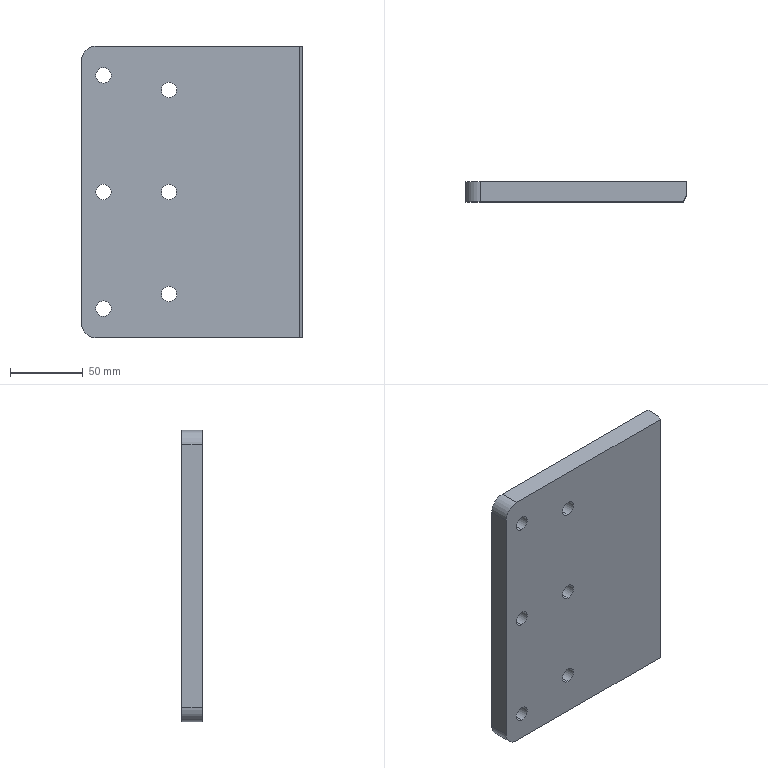Part | SolidWorks | features HoleWzd 2, ICE 2, Extrusion 1, Fillet 1 | 1 solid | 21 faces | box 151.5 x 14 x 200 mm | volume 415411 mm3 | cylinder 14 | plane 7 | commonest cylinder face diameters 10.5 x12 20 x2
STEP:
#1=CARTESIAN_POINT('',(15.,0.,-85.25));
#2=VERTEX_POINT('',#1);
#3=CARTESIAN_POINT('',(15.,0.,-74.75));
#4=VERTEX_POINT('',#3);
#5=CARTESIAN_POINT('',(15.,0.,-80.));
#6=DIRECTION('',(0.,1.,0.));
#7=DIRECTION('',(0.,0.,1.));
#8=AXIS2_PLACEMENT_3D('',#5,#6,#7);
#9=CIRCLE('',#8,5.25);
#10=EDGE_CURVE('',#2,#4,#9,.T.);
#11=ORIENTED_EDGE('',*,*,#10,.F.);
#12=CARTESIAN_POINT('',(15.,14.,-85.25));
#13=VERTEX_POINT('',#12);
#14=CARTESIAN_POINT('',(15.,14.,-85.25));
#15=DIRECTION('',(0.,1.,0.));
#16=VECTOR('',#15,1000.);
#17=LINE('',#14,#16);
#18=EDGE_CURVE('',#2,#13,#17,.T.);
#19=ORIENTED_EDGE('',*,*,#18,.T.);
#20=CARTESIAN_POINT('',(15.,14.,-74.75));
#21=VERTEX_POINT('',#20);
#22=CARTESIAN_POINT('',(15.,14.,-80.));
#23=DIRECTION('',(0.,1.,0.));
#24=DIRECTION('',(0.,0.,1.));
#25=AXIS2_PLACEMENT_3D('',#22,#23,#24);
#26=CIRCLE('',#25,5.25);
#27=EDGE_CURVE('',#13,#21,#26,.T.);
#28=ORIENTED_EDGE('',*,*,#27,.T.);
#29=CARTESIAN_POINT('',(15.,14.,-74.75));
#30=DIRECTION('',(0.,1.,0.));
#31=VECTOR('',#30,1000.);
#32=LINE('',#29,#31);
#33=EDGE_CURVE('',#4,#21,#32,.T.);
#34=ORIENTED_EDGE('',*,*,#33,.F.);
#35=EDGE_LOOP('',(#11,#19,#28,#34));
#36=FACE_OUTER_BOUND('',#35,.T.);
#37=CARTESIAN_POINT('',(15.,14.,-80.));
#38=DIRECTION('',(0.,1.,0.));
#39=DIRECTION('',(0.,0.,1.));
#40=AXIS2_PLACEMENT_3D('',#37,#38,#39);
#41=CYLINDRICAL_SURFACE('',#40,5.25);
#42=ADVANCED_FACE('',(#36),#41,.F.);
#43=CARTESIAN_POINT('',(15.,0.,74.75));
#44=VERTEX_POINT('',#43);
#45=CARTESIAN_POINT('',(15.,0.,85.25));
#46=VERTEX_POINT('',#45);
#47=CARTESIAN_POINT('',(15.,0.,80.));
#48=DIRECTION('',(0.,1.,0.));
#49=DIRECTION('',(0.,0.,1.));
#50=AXIS2_PLACEMENT_3D('',#47,#48,#49);
#51=CIRCLE('',#50,5.25);
#52=EDGE_CURVE('',#44,#46,#51,.T.);
#53=ORIENTED_EDGE('',*,*,#52,.F.);
#54=CARTESIAN_POINT('',(15.,14.,74.75));
#55=VERTEX_POINT('',#54);
#56=CARTESIAN_POINT('',(15.,14.,74.75));
#57=DIRECTION('',(0.,1.,0.));
#58=VECTOR('',#57,1000.);
#59=LINE('',#56,#58);
#60=EDGE_CURVE('',#44,#55,#59,.T.);
#61=ORIENTED_EDGE('',*,*,#60,.T.);
#62=CARTESIAN_POINT('',(15.,14.,85.25));
#63=VERTEX_POINT('',#62);
#64=CARTESIAN_POINT('',(15.,14.,80.));
#65=DIRECTION('',(0.,1.,0.));
#66=DIRECTION('',(0.,0.,1.));
#67=AXIS2_PLACEMENT_3D('',#64,#65,#66);
#68=CIRCLE('',#67,5.25);
#69=EDGE_CURVE('',#55,#63,#68,.T.);
#70=ORIENTED_EDGE('',*,*,#69,.T.);
#71=CARTESIAN_POINT('',(15.,14.,85.25));
#72=DIRECTION('',(0.,1.,0.));
#73=VECTOR('',#72,1000.);
#74=LINE('',#71,#73);
#75=EDGE_CURVE('',#46,#63,#74,.T.);
#76=ORIENTED_EDGE('',*,*,#75,.F.);
#77=EDGE_LOOP('',(#53,#61,#70,#76));
#78=FACE_OUTER_BOUND('',#77,.T.);
#79=CARTESIAN_POINT('',(15.,14.,80.));
#80=DIRECTION('',(0.,1.,0.));
#81=DIRECTION('',(0.,0.,1.));
#82=AXIS2_PLACEMENT_3D('',#79,#80,#81);
#83=CYLINDRICAL_SURFACE('',#82,5.25);
#84=ADVANCED_FACE('',(#78),#83,.F.);
#85=CARTESIAN_POINT('',(15.,0.,-5.25));
#86=VERTEX_POINT('',#85);
#87=CARTESIAN_POINT('',(15.,0.,5.25));
#88=VERTEX_POINT('',#87);
#89=CARTESIAN_POINT('',(15.,0.,0.));
#90=DIRECTION('',(0.,1.,0.));
#91=DIRECTION('',(0.,0.,1.));
#92=AXIS2_PLACEMENT_3D('',#89,#90,#91);
#93=CIRCLE('',#92,5.25);
#94=EDGE_CURVE('',#86,#88,#93,.T.);
#95=ORIENTED_EDGE('',*,*,#94,.F.);
#96=CARTESIAN_POINT('',(15.,14.,-5.25));
#97=VERTEX_POINT('',#96);
#98=CARTESIAN_POINT('',(15.,14.,-5.25));
#99=DIRECTION('',(0.,1.,0.));
#100=VECTOR('',#99,1000.);
#101=LINE('',#98,#100);
#102=EDGE_CURVE('',#86,#97,#101,.T.);
#103=ORIENTED_EDGE('',*,*,#102,.T.);
#104=CARTESIAN_POINT('',(15.,14.,5.25));
#105=VERTEX_POINT('',#104);
#106=CARTESIAN_POINT('',(15.,14.,0.));
#107=DIRECTION('',(0.,1.,0.));
#108=DIRECTION('',(0.,0.,1.));
#109=AXIS2_PLACEMENT_3D('',#106,#107,#108);
#110=CIRCLE('',#109,5.25);
#111=EDGE_CURVE('',#97,#105,#110,.T.);
#112=ORIENTED_EDGE('',*,*,#111,.T.);
#113=CARTESIAN_POINT('',(15.,14.,5.25));
#114=DIRECTION('',(0.,1.,0.));
#115=VECTOR('',#114,1000.);
#116=LINE('',#113,#115);
#117=EDGE_CURVE('',#88,#105,#116,.T.);
#118=ORIENTED_EDGE('',*,*,#117,.F.);
#119=EDGE_LOOP('',(#95,#103,#112,#118));
#120=FACE_OUTER_BOUND('',#119,.T.);
#121=CARTESIAN_POINT('',(15.,14.,0.));
#122=DIRECTION('',(0.,1.,0.));
#123=DIRECTION('',(0.,0.,1.));
#124=AXIS2_PLACEMENT_3D('',#121,#122,#123);
#125=CYLINDRICAL_SURFACE('',#124,5.25);
#126=ADVANCED_FACE('',(#120),#125,.F.);
#127=CARTESIAN_POINT('',(60.,0.,-75.25));
#128=VERTEX_POINT('',#127);
#129=CARTESIAN_POINT('',(60.,0.,-64.75));
#130=VERTEX_POINT('',#129);
#131=CARTESIAN_POINT('',(60.,0.,-70.));
#132=DIRECTION('',(0.,1.,0.));
#133=DIRECTION('',(0.,0.,1.));
#134=AXIS2_PLACEMENT_3D('',#131,#132,#133);
#135=CIRCLE('',#134,5.25);
#136=EDGE_CURVE('',#128,#130,#135,.T.);
#137=ORIENTED_EDGE('',*,*,#136,.F.);
#138=CARTESIAN_POINT('',(60.,14.,-75.25));
#139=VERTEX_POINT('',#138);
#140=CARTESIAN_POINT('',(60.,14.,-75.25));
#141=DIRECTION('',(0.,1.,0.));
#142=VECTOR('',#141,1000.);
#143=LINE('',#140,#142);
#144=EDGE_CURVE('',#128,#139,#143,.T.);
#145=ORIENTED_EDGE('',*,*,#144,.T.);
#146=CARTESIAN_POINT('',(60.,14.,-64.75));
#147=VERTEX_POINT('',#146);
#148=CARTESIAN_POINT('',(60.,14.,-70.));
#149=DIRECTION('',(0.,1.,0.));
#150=DIRECTION('',(0.,0.,1.));
#151=AXIS2_PLACEMENT_3D('',#148,#149,#150);
#152=CIRCLE('',#151,5.25);
#153=EDGE_CURVE('',#139,#147,#152,.T.);
#154=ORIENTED_EDGE('',*,*,#153,.T.);
#155=CARTESIAN_POINT('',(60.,14.,-64.75));
#156=DIRECTION('',(0.,1.,0.));
#157=VECTOR('',#156,1000.);
#158=LINE('',#155,#157);
#159=EDGE_CURVE('',#130,#147,#158,.T.);
#160=ORIENTED_EDGE('',*,*,#159,.F.);
#161=EDGE_LOOP('',(#137,#145,#154,#160));
#162=FACE_OUTER_BOUND('',#161,.T.);
#163=CARTESIAN_POINT('',(60.,14.,-70.));
#164=DIRECTION('',(0.,1.,0.));
#165=DIRECTION('',(0.,0.,1.));
#166=AXIS2_PLACEMENT_3D('',#163,#164,#165);
#167=CYLINDRICAL_SURFACE('',#166,5.25);
#168=ADVANCED_FACE('',(#162),#167,.F.);
#169=CARTESIAN_POINT('',(60.,0.,64.75));
#170=VERTEX_POINT('',#169);
#171=CARTESIAN_POINT('',(60.,0.,75.25));
#172=VERTEX_POINT('',#171);
#173=CARTESIAN_POINT('',(60.,0.,70.));
#174=DIRECTION('',(0.,1.,0.));
#175=DIRECTION('',(0.,0.,1.));
#176=AXIS2_PLACEMENT_3D('',#173,#174,#175);
#177=CIRCLE('',#176,5.25);
#178=EDGE_CURVE('',#170,#172,#177,.T.);
#179=ORIENTED_EDGE('',*,*,#178,.F.);
#180=CARTESIAN_POINT('',(60.,14.,64.75));
#181=VERTEX_POINT('',#180);
#182=CARTESIAN_POINT('',(60.,14.,64.75));
#183=DIRECTION('',(0.,1.,0.));
#184=VECTOR('',#183,1000.);
#185=LINE('',#182,#184);
#186=EDGE_CURVE('',#170,#181,#185,.T.);
#187=ORIENTED_EDGE('',*,*,#186,.T.);
#188=CARTESIAN_POINT('',(60.,14.,75.25));
#189=VERTEX_POINT('',#188);
#190=CARTESIAN_POINT('',(60.,14.,70.));
#191=DIRECTION('',(0.,1.,0.));
#192=DIRECTION('',(0.,0.,1.));
#193=AXIS2_PLACEMENT_3D('',#190,#191,#192);
#194=CIRCLE('',#193,5.25);
#195=EDGE_CURVE('',#181,#189,#194,.T.);
#196=ORIENTED_EDGE('',*,*,#195,.T.);
#197=CARTESIAN_POINT('',(60.,14.,75.25));
#198=DIRECTION('',(0.,1.,0.));
#199=VECTOR('',#198,1000.);
#200=LINE('',#197,#199);
#201=EDGE_CURVE('',#172,#189,#200,.T.);
#202=ORIENTED_EDGE('',*,*,#201,.F.);
#203=EDGE_LOOP('',(#179,#187,#196,#202));
#204=FACE_OUTER_BOUND('',#203,.T.);
#205=CARTESIAN_POINT('',(60.,14.,70.));
#206=DIRECTION('',(0.,1.,0.));
#207=DIRECTION('',(0.,0.,1.));
#208=AXIS2_PLACEMENT_3D('',#205,#206,#207);
#209=CYLINDRICAL_SURFACE('',#208,5.25);
#210=ADVANCED_FACE('',(#204),#209,.F.);
#211=CARTESIAN_POINT('',(60.,0.,-5.25));
#212=VERTEX_POINT('',#211);
#213=CARTESIAN_POINT('',(60.,0.,5.25));
#214=VERTEX_POINT('',#213);
#215=CARTESIAN_POINT('',(60.,0.,0.));
#216=DIRECTION('',(0.,1.,0.));
#217=DIRECTION('',(0.,0.,1.));
#218=AXIS2_PLACEMENT_3D('',#215,#216,#217);
#219=CIRCLE('',#218,5.25);
#220=EDGE_CURVE('',#212,#214,#219,.T.);
#221=ORIENTED_EDGE('',*,*,#220,.F.);
#222=CARTESIAN_POINT('',(60.,14.,-5.25));
#223=VERTEX_POINT('',#222);
#224=CARTESIAN_POINT('',(60.,14.,-5.25));
#225=DIRECTION('',(0.,1.,0.));
#226=VECTOR('',#225,1000.);
#227=LINE('',#224,#226);
#228=EDGE_CURVE('',#212,#223,#227,.T.);
#229=ORIENTED_EDGE('',*,*,#228,.T.);
#230=CARTESIAN_POINT('',(60.,14.,5.25));
#231=VERTEX_POINT('',#230);
#232=CARTESIAN_POINT('',(60.,14.,0.));
#233=DIRECTION('',(0.,1.,0.));
#234=DIRECTION('',(0.,0.,1.));
#235=AXIS2_PLACEMENT_3D('',#232,#233,#234);
#236=CIRCLE('',#235,5.25);
#237=EDGE_CURVE('',#223,#231,#236,.T.);
#238=ORIENTED_EDGE('',*,*,#237,.T.);
#239=CARTESIAN_POINT('',(60.,14.,5.25));
#240=DIRECTION('',(0.,1.,0.));
#241=VECTOR('',#240,1000.);
#242=LINE('',#239,#241);
#243=EDGE_CURVE('',#214,#231,#242,.T.);
#244=ORIENTED_EDGE('',*,*,#243,.F.);
#245=EDGE_LOOP('',(#221,#229,#238,#244));
#246=FACE_OUTER_BOUND('',#245,.T.);
#247=CARTESIAN_POINT('',(60.,14.,0.));
#248=DIRECTION('',(0.,1.,0.));
#249=DIRECTION('',(0.,0.,1.));
#250=AXIS2_PLACEMENT_3D('',#247,#248,#249);
#251=CYLINDRICAL_SURFACE('',#250,5.25);
#252=ADVANCED_FACE('',(#246),#251,.F.);
#253=CARTESIAN_POINT('',(0.,14.,-90.));
#254=VERTEX_POINT('',#253);
#255=CARTESIAN_POINT('',(0.,14.,90.));
#256=VERTEX_POINT('',#255);
#257=CARTESIAN_POINT('',(0.,14.,100.));
#258=DIRECTION('',(0.,0.,1.));
#259=VECTOR('',#258,1000.);
#260=LINE('',#257,#259);
#261=EDGE_CURVE('',#254,#256,#260,.T.);
#262=ORIENTED_EDGE('',*,*,#261,.F.);
#263=CARTESIAN_POINT('',(0.,0.,-90.));
#264=VERTEX_POINT('',#263);
#265=CARTESIAN_POINT('',(0.,14.,-90.));
#266=DIRECTION('',(0.,-1.,0.));
#267=VECTOR('',#266,1000.);
#268=LINE('',#265,#267);
#269=EDGE_CURVE('',#254,#264,#268,.T.);
#270=ORIENTED_EDGE('',*,*,#269,.T.);
#271=CARTESIAN_POINT('',(0.,0.,90.));
#272=VERTEX_POINT('',#271);
#273=CARTESIAN_POINT('',(0.,0.,100.));
#274=DIRECTION('',(0.,0.,1.));
#275=VECTOR('',#274,1000.);
#276=LINE('',#273,#275);
#277=EDGE_CURVE('',#264,#272,#276,.T.);
#278=ORIENTED_EDGE('',*,*,#277,.T.);
#279=CARTESIAN_POINT('',(0.,14.,90.));
#280=DIRECTION('',(0.,1.,0.));
#281=VECTOR('',#280,1000.);
#282=LINE('',#279,#281);
#283=EDGE_CURVE('',#272,#256,#282,.T.);
#284=ORIENTED_EDGE('',*,*,#283,.T.);
#285=EDGE_LOOP('',(#262,#270,#278,#284));
#286=FACE_OUTER_BOUND('',#285,.T.);
#287=CARTESIAN_POINT('',(0.,14.,100.));
#288=DIRECTION('',(1.,0.,0.));
#289=DIRECTION('',(0.,0.,-1.));
#290=AXIS2_PLACEMENT_3D('',#287,#288,#289);
#291=PLANE('',#290);
#292=ADVANCED_FACE('',(#286),#291,.F.);
#293=CARTESIAN_POINT('',(151.5,4.429,100.));
#294=VERTEX_POINT('',#293);
#295=CARTESIAN_POINT('',(149.435,0.,100.));
#296=VERTEX_POINT('',#295);
#297=CARTESIAN_POINT('',(149.435,0.,100.));
#298=DIRECTION('',(-0.4226,-0.9063,0.));
#299=VECTOR('',#298,1000.);
#300=LINE('',#297,#299);
#301=EDGE_CURVE('',#294,#296,#300,.T.);
#302=ORIENTED_EDGE('',*,*,#301,.F.);
#303=CARTESIAN_POINT('',(151.5,14.,100.));
#304=VERTEX_POINT('',#303);
#305=CARTESIAN_POINT('',(151.5,14.,100.));
#306=DIRECTION('',(0.,-1.,0.));
#307=VECTOR('',#306,1000.);
#308=LINE('',#305,#307);
#309=EDGE_CURVE('',#304,#294,#308,.T.);
#310=ORIENTED_EDGE('',*,*,#309,.F.);
#311=CARTESIAN_POINT('',(10.,14.,100.));
#312=VERTEX_POINT('',#311);
#313=CARTESIAN_POINT('',(0.,14.,100.));
#314=DIRECTION('',(1.,0.,0.));
#315=VECTOR('',#314,1000.);
#316=LINE('',#313,#315);
#317=EDGE_CURVE('',#312,#304,#316,.T.);
#318=ORIENTED_EDGE('',*,*,#317,.F.);
#319=CARTESIAN_POINT('',(10.,0.,100.));
#320=VERTEX_POINT('',#319);
#321=CARTESIAN_POINT('',(10.,14.,100.));
#322=DIRECTION('',(0.,-1.,0.));
#323=VECTOR('',#322,1000.);
#324=LINE('',#321,#323);
#325=EDGE_CURVE('',#312,#320,#324,.T.);
#326=ORIENTED_EDGE('',*,*,#325,.T.);
#327=CARTESIAN_POINT('',(80.,0.,100.));
#328=DIRECTION('',(1.,0.,0.));
#329=VECTOR('',#328,1000.);
#330=LINE('',#327,#329);
#331=EDGE_CURVE('',#320,#296,#330,.T.);
#332=ORIENTED_EDGE('',*,*,#331,.T.);
#333=EDGE_LOOP('',(#302,#310,#318,#326,#332));
#334=FACE_OUTER_BOUND('',#333,.T.);
#335=CARTESIAN_POINT('',(80.,14.,100.));
#336=DIRECTION('',(0.,0.,-1.));
#337=DIRECTION('',(-1.,0.,0.));
#338=AXIS2_PLACEMENT_3D('',#335,#336,#337);
#339=PLANE('',#338);
#340=ADVANCED_FACE('',(#334),#339,.F.);
#341=CARTESIAN_POINT('',(151.5,14.,-100.));
#342=VERTEX_POINT('',#341);
#343=CARTESIAN_POINT('',(10.,14.,-100.));
#344=VERTEX_POINT('',#343);
#345=CARTESIAN_POINT('',(0.,14.,-100.));
#346=DIRECTION('',(-1.,0.,0.));
#347=VECTOR('',#346,1000.);
#348=LINE('',#345,#347);
#349=EDGE_CURVE('',#342,#344,#348,.T.);
#350=ORIENTED_EDGE('',*,*,#349,.F.);
#351=CARTESIAN_POINT('',(151.5,4.429,-100.));
#352=VERTEX_POINT('',#351);
#353=CARTESIAN_POINT('',(151.5,14.,-100.));
#354=DIRECTION('',(0.,-1.,0.));
#355=VECTOR('',#354,1000.);
#356=LINE('',#353,#355);
#357=EDGE_CURVE('',#342,#352,#356,.T.);
#358=ORIENTED_EDGE('',*,*,#357,.T.);
#359=CARTESIAN_POINT('',(149.435,0.,-100.));
#360=VERTEX_POINT('',#359);
#361=CARTESIAN_POINT('',(149.435,0.,-100.));
#362=DIRECTION('',(-0.4226,-0.9063,0.));
#363=VECTOR('',#362,1000.);
#364=LINE('',#361,#363);
#365=EDGE_CURVE('',#352,#360,#364,.T.);
#366=ORIENTED_EDGE('',*,*,#365,.T.);
#367=CARTESIAN_POINT('',(10.,0.,-100.));
#368=VERTEX_POINT('',#367);
#369=CARTESIAN_POINT('',(80.,0.,-100.));
#370=DIRECTION('',(-1.,0.,0.));
#371=VECTOR('',#370,1000.);
#372=LINE('',#369,#371);
#373=EDGE_CURVE('',#360,#368,#372,.T.);
#374=ORIENTED_EDGE('',*,*,#373,.T.);
#375=CARTESIAN_POINT('',(10.,14.,-100.));
#376=DIRECTION('',(0.,1.,0.));
#377=VECTOR('',#376,1000.);
#378=LINE('',#375,#377);
#379=EDGE_CURVE('',#368,#344,#378,.T.);
#380=ORIENTED_EDGE('',*,*,#379,.T.);
#381=EDGE_LOOP('',(#350,#358,#366,#374,#380));
#382=FACE_OUTER_BOUND('',#381,.T.);
#383=CARTESIAN_POINT('',(80.,14.,-100.));
#384=DIRECTION('',(0.,0.,1.));
#385=DIRECTION('',(1.,0.,0.));
#386=AXIS2_PLACEMENT_3D('',#383,#384,#385);
#387=PLANE('',#386);
#388=ADVANCED_FACE('',(#382),#387,.F.);
#389=CARTESIAN_POINT('',(15.,14.,-80.));
#390=DIRECTION('',(0.,1.,0.));
#391=DIRECTION('',(0.,0.,1.));
#392=AXIS2_PLACEMENT_3D('',#389,#390,#391);
#393=CIRCLE('',#392,5.25);
#394=EDGE_CURVE('',#21,#13,#393,.T.);
#395=ORIENTED_EDGE('',*,*,#394,.F.);
#396=ORIENTED_EDGE('',*,*,#27,.F.);
#397=EDGE_LOOP('',(#395,#396));
#398=FACE_BOUND('',#397,.T.);
#399=CARTESIAN_POINT('',(15.,14.,80.));
#400=DIRECTION('',(0.,1.,0.));
#401=DIRECTION('',(0.,0.,1.));
#402=AXIS2_PLACEMENT_3D('',#399,#400,#401);
#403=CIRCLE('',#402,5.25);
#404=EDGE_CURVE('',#63,#55,#403,.T.);
#405=ORIENTED_EDGE('',*,*,#404,.F.);
#406=ORIENTED_EDGE('',*,*,#69,.F.);
#407=EDGE_LOOP('',(#405,#406));
#408=FACE_BOUND('',#407,.T.);
#409=CARTESIAN_POINT('',(15.,14.,0.));
#410=DIRECTION('',(0.,1.,0.));
#411=DIRECTION('',(0.,0.,1.));
#412=AXIS2_PLACEMENT_3D('',#409,#410,#411);
#413=CIRCLE('',#412,5.25);
#414=EDGE_CURVE('',#105,#97,#413,.T.);
#415=ORIENTED_EDGE('',*,*,#414,.F.);
#416=ORIENTED_EDGE('',*,*,#111,.F.);
#417=EDGE_LOOP('',(#415,#416));
#418=FACE_BOUND('',#417,.T.);
#419=CARTESIAN_POINT('',(60.,14.,-70.));
#420=DIRECTION('',(0.,1.,0.));
#421=DIRECTION('',(0.,0.,1.));
#422=AXIS2_PLACEMENT_3D('',#419,#420,#421);
#423=CIRCLE('',#422,5.25);
#424=EDGE_CURVE('',#147,#139,#423,.T.);
#425=ORIENTED_EDGE('',*,*,#424,.F.);
#426=ORIENTED_EDGE('',*,*,#153,.F.);
#427=EDGE_LOOP('',(#425,#426));
#428=FACE_BOUND('',#427,.T.);
#429=CARTESIAN_POINT('',(60.,14.,70.));
#430=DIRECTION('',(0.,1.,0.));
#431=DIRECTION('',(0.,0.,1.));
#432=AXIS2_PLACEMENT_3D('',#429,#430,#431);
#433=CIRCLE('',#432,5.25);
#434=EDGE_CURVE('',#189,#181,#433,.T.);
#435=ORIENTED_EDGE('',*,*,#434,.F.);
#436=ORIENTED_EDGE('',*,*,#195,.F.);
#437=EDGE_LOOP('',(#435,#436));
#438=FACE_BOUND('',#437,.T.);
#439=CARTESIAN_POINT('',(60.,14.,0.));
#440=DIRECTION('',(0.,1.,0.));
#441=DIRECTION('',(0.,0.,1.));
#442=AXIS2_PLACEMENT_3D('',#439,#440,#441);
#443=CIRCLE('',#442,5.25);
#444=EDGE_CURVE('',#231,#223,#443,.T.);
#445=ORIENTED_EDGE('',*,*,#444,.F.);
#446=ORIENTED_EDGE('',*,*,#237,.F.);
#447=EDGE_LOOP('',(#445,#446));
#448=FACE_BOUND('',#447,.T.);
#449=ORIENTED_EDGE('',*,*,#317,.T.);
#450=CARTESIAN_POINT('',(151.5,14.,-100.));
#451=DIRECTION('',(0.,0.,1.));
#452=VECTOR('',#451,1000.);
#453=LINE('',#450,#452);
#454=EDGE_CURVE('',#342,#304,#453,.T.);
#455=ORIENTED_EDGE('',*,*,#454,.F.);
#456=ORIENTED_EDGE('',*,*,#349,.T.);
#457=CARTESIAN_POINT('',(10.,14.,-90.));
#458=DIRECTION('',(0.,1.,0.));
#459=DIRECTION('',(0.,0.,-1.));
#460=AXIS2_PLACEMENT_3D('',#457,#458,#459);
#461=CIRCLE('',#460,10.);
#462=EDGE_CURVE('',#344,#254,#461,.T.);
#463=ORIENTED_EDGE('',*,*,#462,.T.);
#464=ORIENTED_EDGE('',*,*,#261,.T.);
#465=CARTESIAN_POINT('',(10.,14.,90.));
#466=DIRECTION('',(0.,1.,0.));
#467=DIRECTION('',(0.,0.,-1.));
#468=AXIS2_PLACEMENT_3D('',#465,#466,#467);
#469=CIRCLE('',#468,10.);
#470=EDGE_CURVE('',#256,#312,#469,.T.);
#471=ORIENTED_EDGE('',*,*,#470,.T.);
#472=EDGE_LOOP('',(#449,#455,#456,#463,#464,#471));
#473=FACE_OUTER_BOUND('',#472,.T.);
#474=CARTESIAN_POINT('',(0.,14.,0.));
#475=DIRECTION('',(0.,-1.,0.));
#476=DIRECTION('',(0.,0.,-1.));
#477=AXIS2_PLACEMENT_3D('',#474,#475,#476);
#478=PLANE('',#477);
#479=ADVANCED_FACE('',(#398,#408,#418,#428,#438,#448,#473),#478,.F.);
#480=CARTESIAN_POINT('',(149.435,0.,-100.));
#481=DIRECTION('',(0.,0.,1.));
#482=VECTOR('',#481,1000.);
#483=LINE('',#480,#482);
#484=EDGE_CURVE('',#360,#296,#483,.T.);
#485=ORIENTED_EDGE('',*,*,#484,.T.);
#486=ORIENTED_EDGE('',*,*,#331,.F.);
#487=CARTESIAN_POINT('',(10.,0.,90.));
#488=DIRECTION('',(0.,-1.,0.));
#489=DIRECTION('',(0.,0.,-1.));
#490=AXIS2_PLACEMENT_3D('',#487,#488,#489);
#491=CIRCLE('',#490,10.);
#492=EDGE_CURVE('',#320,#272,#491,.T.);
#493=ORIENTED_EDGE('',*,*,#492,.T.);
#494=ORIENTED_EDGE('',*,*,#277,.F.);
#495=CARTESIAN_POINT('',(10.,0.,-90.));
#496=DIRECTION('',(0.,-1.,0.));
#497=DIRECTION('',(0.,0.,-1.));
#498=AXIS2_PLACEMENT_3D('',#495,#496,#497);
#499=CIRCLE('',#498,10.);
#500=EDGE_CURVE('',#264,#368,#499,.T.);
#501=ORIENTED_EDGE('',*,*,#500,.T.);
#502=ORIENTED_EDGE('',*,*,#373,.F.);
#503=EDGE_LOOP('',(#485,#486,#493,#494,#501,#502));
#504=FACE_OUTER_BOUND('',#503,.T.);
#505=CARTESIAN_POINT('',(15.,0.,-80.));
#506=DIRECTION('',(0.,1.,0.));
#507=DIRECTION('',(0.,0.,1.));
#508=AXIS2_PLACEMENT_3D('',#505,#506,#507);
#509=CIRCLE('',#508,5.25);
#510=EDGE_CURVE('',#4,#2,#509,.T.);
#511=ORIENTED_EDGE('',*,*,#510,.T.);
#512=ORIENTED_EDGE('',*,*,#10,.T.);
#513=EDGE_LOOP('',(#511,#512));
#514=FACE_BOUND('',#513,.T.);
#515=CARTESIAN_POINT('',(15.,0.,80.));
#516=DIRECTION('',(0.,1.,0.));
#517=DIRECTION('',(0.,0.,1.));
#518=AXIS2_PLACEMENT_3D('',#515,#516,#517);
#519=CIRCLE('',#518,5.25);
#520=EDGE_CURVE('',#46,#44,#519,.T.);
#521=ORIENTED_EDGE('',*,*,#520,.T.);
#522=ORIENTED_EDGE('',*,*,#52,.T.);
#523=EDGE_LOOP('',(#521,#522));
#524=FACE_BOUND('',#523,.T.);
#525=CARTESIAN_POINT('',(15.,0.,0.));
#526=DIRECTION('',(0.,1.,0.));
#527=DIRECTION('',(0.,0.,1.));
#528=AXIS2_PLACEMENT_3D('',#525,#526,#527);
#529=CIRCLE('',#528,5.25);
#530=EDGE_CURVE('',#88,#86,#529,.T.);
#531=ORIENTED_EDGE('',*,*,#530,.T.);
#532=ORIENTED_EDGE('',*,*,#94,.T.);
#533=EDGE_LOOP('',(#531,#532));
#534=FACE_BOUND('',#533,.T.);
#535=CARTESIAN_POINT('',(60.,0.,-70.));
#536=DIRECTION('',(0.,1.,0.));
#537=DIRECTION('',(0.,0.,1.));
#538=AXIS2_PLACEMENT_3D('',#535,#536,#537);
#539=CIRCLE('',#538,5.25);
#540=EDGE_CURVE('',#130,#128,#539,.T.);
#541=ORIENTED_EDGE('',*,*,#540,.T.);
#542=ORIENTED_EDGE('',*,*,#136,.T.);
#543=EDGE_LOOP('',(#541,#542));
#544=FACE_BOUND('',#543,.T.);
#545=CARTESIAN_POINT('',(60.,0.,70.));
#546=DIRECTION('',(0.,1.,0.));
#547=DIRECTION('',(0.,0.,1.));
#548=AXIS2_PLACEMENT_3D('',#545,#546,#547);
#549=CIRCLE('',#548,5.25);
#550=EDGE_CURVE('',#172,#170,#549,.T.);
#551=ORIENTED_EDGE('',*,*,#550,.T.);
#552=ORIENTED_EDGE('',*,*,#178,.T.);
#553=EDGE_LOOP('',(#551,#552));
#554=FACE_BOUND('',#553,.T.);
#555=CARTESIAN_POINT('',(60.,0.,0.));
#556=DIRECTION('',(0.,1.,0.));
#557=DIRECTION('',(0.,0.,1.));
#558=AXIS2_PLACEMENT_3D('',#555,#556,#557);
#559=CIRCLE('',#558,5.25);
#560=EDGE_CURVE('',#214,#212,#559,.T.);
#561=ORIENTED_EDGE('',*,*,#560,.T.);
#562=ORIENTED_EDGE('',*,*,#220,.T.);
#563=EDGE_LOOP('',(#561,#562));
#564=FACE_BOUND('',#563,.T.);
#565=CARTESIAN_POINT('',(0.,0.,0.));
#566=DIRECTION('',(0.,-1.,0.));
#567=DIRECTION('',(0.,0.,-1.));
#568=AXIS2_PLACEMENT_3D('',#565,#566,#567);
#569=PLANE('',#568);
#570=ADVANCED_FACE('',(#504,#514,#524,#534,#544,#554,#564),#569,.T.);
#571=ORIENTED_EDGE('',*,*,#462,.F.);
#572=ORIENTED_EDGE('',*,*,#379,.F.);
#573=ORIENTED_EDGE('',*,*,#500,.F.);
#574=ORIENTED_EDGE('',*,*,#269,.F.);
#575=EDGE_LOOP('',(#571,#572,#573,#574));
#576=FACE_OUTER_BOUND('',#575,.T.);
#577=CARTESIAN_POINT('',(10.,14.,-90.));
#578=DIRECTION('',(0.,-1.,0.));
#579=DIRECTION('',(0.,0.,-1.));
#580=AXIS2_PLACEMENT_3D('',#577,#578,#579);
#581=CYLINDRICAL_SURFACE('',#580,10.);
#582=ADVANCED_FACE('',(#576),#581,.T.);
#583=ORIENTED_EDGE('',*,*,#470,.F.);
#584=ORIENTED_EDGE('',*,*,#283,.F.);
#585=ORIENTED_EDGE('',*,*,#492,.F.);
#586=ORIENTED_EDGE('',*,*,#325,.F.);
#587=EDGE_LOOP('',(#583,#584,#585,#586));
#588=FACE_OUTER_BOUND('',#587,.T.);
#589=CARTESIAN_POINT('',(10.,14.,90.));
#590=DIRECTION('',(0.,-1.,0.));
#591=DIRECTION('',(0.,0.,-1.));
#592=AXIS2_PLACEMENT_3D('',#589,#590,#591);
#593=CYLINDRICAL_SURFACE('',#592,10.);
#594=ADVANCED_FACE('',(#588),#593,.T.);
#595=ORIENTED_EDGE('',*,*,#228,.F.);
#596=ORIENTED_EDGE('',*,*,#560,.F.);
#597=ORIENTED_EDGE('',*,*,#243,.T.);
#598=ORIENTED_EDGE('',*,*,#444,.T.);
#599=EDGE_LOOP('',(#595,#596,#597,#598));
#600=FACE_OUTER_BOUND('',#599,.T.);
#601=CARTESIAN_POINT('',(60.,14.,0.));
#602=DIRECTION('',(0.,1.,0.));
#603=DIRECTION('',(0.,0.,1.));
#604=AXIS2_PLACEMENT_3D('',#601,#602,#603);
#605=CYLINDRICAL_SURFACE('',#604,5.25);
#606=ADVANCED_FACE('',(#600),#605,.F.);
#607=ORIENTED_EDGE('',*,*,#186,.F.);
#608=ORIENTED_EDGE('',*,*,#550,.F.);
#609=ORIENTED_EDGE('',*,*,#201,.T.);
#610=ORIENTED_EDGE('',*,*,#434,.T.);
#611=EDGE_LOOP('',(#607,#608,#609,#610));
#612=FACE_OUTER_BOUND('',#611,.T.);
#613=CARTESIAN_POINT('',(60.,14.,70.));
#614=DIRECTION('',(0.,1.,0.));
#615=DIRECTION('',(0.,0.,1.));
#616=AXIS2_PLACEMENT_3D('',#613,#614,#615);
#617=CYLINDRICAL_SURFACE('',#616,5.25);
#618=ADVANCED_FACE('',(#612),#617,.F.);
#619=ORIENTED_EDGE('',*,*,#144,.F.);
#620=ORIENTED_EDGE('',*,*,#540,.F.);
#621=ORIENTED_EDGE('',*,*,#159,.T.);
#622=ORIENTED_EDGE('',*,*,#424,.T.);
#623=EDGE_LOOP('',(#619,#620,#621,#622));
#624=FACE_OUTER_BOUND('',#623,.T.);
#625=CARTESIAN_POINT('',(60.,14.,-70.));
#626=DIRECTION('',(0.,1.,0.));
#627=DIRECTION('',(0.,0.,1.));
#628=AXIS2_PLACEMENT_3D('',#625,#626,#627);
#629=CYLINDRICAL_SURFACE('',#628,5.25);
#630=ADVANCED_FACE('',(#624),#629,.F.);
#631=ORIENTED_EDGE('',*,*,#102,.F.);
#632=ORIENTED_EDGE('',*,*,#530,.F.);
#633=ORIENTED_EDGE('',*,*,#117,.T.);
#634=ORIENTED_EDGE('',*,*,#414,.T.);
#635=EDGE_LOOP('',(#631,#632,#633,#634));
#636=FACE_OUTER_BOUND('',#635,.T.);
#637=CARTESIAN_POINT('',(15.,14.,0.));
#638=DIRECTION('',(0.,1.,0.));
#639=DIRECTION('',(0.,0.,1.));
#640=AXIS2_PLACEMENT_3D('',#637,#638,#639);
#641=CYLINDRICAL_SURFACE('',#640,5.25);
#642=ADVANCED_FACE('',(#636),#641,.F.);
#643=ORIENTED_EDGE('',*,*,#60,.F.);
#644=ORIENTED_EDGE('',*,*,#520,.F.);
#645=ORIENTED_EDGE('',*,*,#75,.T.);
#646=ORIENTED_EDGE('',*,*,#404,.T.);
#647=EDGE_LOOP('',(#643,#644,#645,#646));
#648=FACE_OUTER_BOUND('',#647,.T.);
#649=CARTESIAN_POINT('',(15.,14.,80.));
#650=DIRECTION('',(0.,1.,0.));
#651=DIRECTION('',(0.,0.,1.));
#652=AXIS2_PLACEMENT_3D('',#649,#650,#651);
#653=CYLINDRICAL_SURFACE('',#652,5.25);
#654=ADVANCED_FACE('',(#648),#653,.F.);
#655=ORIENTED_EDGE('',*,*,#18,.F.);
#656=ORIENTED_EDGE('',*,*,#510,.F.);
#657=ORIENTED_EDGE('',*,*,#33,.T.);
#658=ORIENTED_EDGE('',*,*,#394,.T.);
#659=EDGE_LOOP('',(#655,#656,#657,#658));
#660=FACE_OUTER_BOUND('',#659,.T.);
#661=CARTESIAN_POINT('',(15.,14.,-80.));
#662=DIRECTION('',(0.,1.,0.));
#663=DIRECTION('',(0.,0.,1.));
#664=AXIS2_PLACEMENT_3D('',#661,#662,#663);
#665=CYLINDRICAL_SURFACE('',#664,5.25);
#666=ADVANCED_FACE('',(#660),#665,.F.);
#667=ORIENTED_EDGE('',*,*,#365,.F.);
#668=CARTESIAN_POINT('',(151.5,4.429,-100.));
#669=DIRECTION('',(0.,0.,1.));
#670=VECTOR('',#669,1000.);
#671=LINE('',#668,#670);
#672=EDGE_CURVE('',#352,#294,#671,.T.);
#673=ORIENTED_EDGE('',*,*,#672,.T.);
#674=ORIENTED_EDGE('',*,*,#301,.T.);
#675=ORIENTED_EDGE('',*,*,#484,.F.);
#676=EDGE_LOOP('',(#667,#673,#674,#675));
#677=FACE_OUTER_BOUND('',#676,.T.);
#678=CARTESIAN_POINT('',(149.435,0.,-100.));
#679=DIRECTION('',(-0.9063,0.4226,0.));
#680=DIRECTION('',(-0.4226,-0.9063,0.));
#681=AXIS2_PLACEMENT_3D('',#678,#679,#680);
#682=PLANE('',#681);
#683=ADVANCED_FACE('',(#677),#682,.F.);
#684=ORIENTED_EDGE('',*,*,#357,.F.);
#685=ORIENTED_EDGE('',*,*,#454,.T.);
#686=ORIENTED_EDGE('',*,*,#309,.T.);
#687=ORIENTED_EDGE('',*,*,#672,.F.);
#688=EDGE_LOOP('',(#684,#685,#686,#687));
#689=FACE_OUTER_BOUND('',#688,.T.);
#690=CARTESIAN_POINT('',(151.5,14.,-100.));
#691=DIRECTION('',(-1.,0.,0.));
#692=DIRECTION('',(0.,0.,1.));
#693=AXIS2_PLACEMENT_3D('',#690,#691,#692);
#694=PLANE('',#693);
#695=ADVANCED_FACE('',(#689),#694,.F.);
#696=CLOSED_SHELL('',(#42,#84,#126,#168,#210,#252,#292,#340,#388,#479,#570,#582,#594,#606,#618,#630,#642,#654,#666,#683,#695));
#697=MANIFOLD_SOLID_BREP('',#696);
#698=CARTESIAN_POINT('',(0.,0.,0.));
#699=DIRECTION('',(0.,0.,1.));
#700=DIRECTION('',(1.,0.,0.));
#701=AXIS2_PLACEMENT_3D('',#698,#699,#700);
#702=(LENGTH_UNIT()NAMED_UNIT(*)SI_UNIT(.MILLI.,.METRE.));
#703=UNCERTAINTY_MEASURE_WITH_UNIT(LENGTH_MEASURE(0.00001),#702,'','');
#704=(NAMED_UNIT(*)PLANE_ANGLE_UNIT()SI_UNIT($,.RADIAN.));
#705=(NAMED_UNIT(*)SI_UNIT($,.STERADIAN.)SOLID_ANGLE_UNIT());
#706=(GEOMETRIC_REPRESENTATION_CONTEXT(3)GLOBAL_UNCERTAINTY_ASSIGNED_CONTEXT((#703))GLOBAL_UNIT_ASSIGNED_CONTEXT((#702,#704,#705))REPRESENTATION_CONTEXT('',''));
#707=ADVANCED_BREP_SHAPE_REPRESENTATION('',(#697,#701),#706);